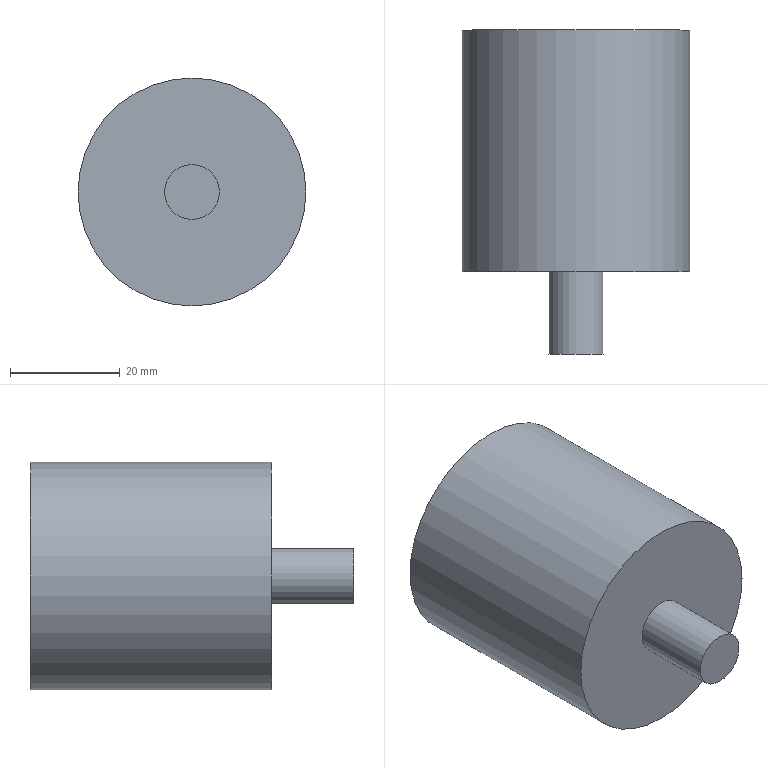Part | STEP file | 冲床-300配套压波_id286_x_t | 1 solid | 5 faces | box 41.5 x 59 x 41.5 mm | volume 60695 mm3 | plane 3 | cylinder 2 | commonest cylinder face diameters 10 x1 41.5 x1
STEP:
#1=CARTESIAN_POINT('',(1130.,22.,181.5));
#2=VERTEX_POINT('',#1);
#3=CARTESIAN_POINT('',(1130.,22.,160.75));
#4=DIRECTION('',(0.,-1.,0.));
#5=DIRECTION('',(0.,0.,1.));
#6=AXIS2_PLACEMENT_3D('',#3,#4,#5);
#7=CIRCLE('',#6,20.75);
#8=EDGE_CURVE('',#2,#2,#7,.T.);
#9=ORIENTED_EDGE('',*,*,#8,.F.);
#10=EDGE_LOOP('',(#9));
#11=FACE_OUTER_BOUND('',#10,.T.);
#12=CARTESIAN_POINT('',(1130.,22.,110.));
#13=DIRECTION('',(0.,1.,0.));
#14=DIRECTION('',(0.,0.,1.));
#15=AXIS2_PLACEMENT_3D('',#12,#13,#14);
#16=PLANE('',#15);
#17=ADVANCED_FACE('',(#11),#16,.T.);
#18=CARTESIAN_POINT('',(1130.,-22.,181.5));
#19=VERTEX_POINT('',#18);
#20=CARTESIAN_POINT('',(1130.,-22.,160.75));
#21=DIRECTION('',(0.,1.,0.));
#22=DIRECTION('',(0.,0.,1.));
#23=AXIS2_PLACEMENT_3D('',#20,#21,#22);
#24=CIRCLE('',#23,20.75);
#25=EDGE_CURVE('',#19,#19,#24,.T.);
#26=ORIENTED_EDGE('',*,*,#25,.T.);
#27=EDGE_LOOP('',(#26));
#28=FACE_BOUND('',#27,.T.);
#29=ORIENTED_EDGE('',*,*,#8,.T.);
#30=EDGE_LOOP('',(#29));
#31=FACE_BOUND('',#30,.T.);
#32=CARTESIAN_POINT('',(1130.,-20.,160.75));
#33=DIRECTION('',(0.,1.,0.));
#34=DIRECTION('',(0.,0.,1.));
#35=AXIS2_PLACEMENT_3D('',#32,#33,#34);
#36=CYLINDRICAL_SURFACE('',#35,20.75);
#37=ADVANCED_FACE('',(#28,#31),#36,.T.);
#38=CARTESIAN_POINT('',(1130.,-22.,155.75));
#39=VERTEX_POINT('',#38);
#40=CARTESIAN_POINT('',(1130.,-22.,160.75));
#41=DIRECTION('',(0.,-1.,0.));
#42=DIRECTION('',(0.,0.,-1.));
#43=AXIS2_PLACEMENT_3D('',#40,#41,#42);
#44=CIRCLE('',#43,5.);
#45=EDGE_CURVE('',#39,#39,#44,.T.);
#46=ORIENTED_EDGE('',*,*,#45,.F.);
#47=EDGE_LOOP('',(#46));
#48=FACE_BOUND('',#47,.T.);
#49=ORIENTED_EDGE('',*,*,#25,.F.);
#50=EDGE_LOOP('',(#49));
#51=FACE_BOUND('',#50,.T.);
#52=CARTESIAN_POINT('',(1130.,-22.,160.75));
#53=DIRECTION('',(0.,1.,0.));
#54=DIRECTION('',(0.,0.,1.));
#55=AXIS2_PLACEMENT_3D('',#52,#53,#54);
#56=PLANE('',#55);
#57=ADVANCED_FACE('',(#48,#51),#56,.F.);
#58=CARTESIAN_POINT('',(1130.,-37.,165.75));
#59=VERTEX_POINT('',#58);
#60=CARTESIAN_POINT('',(1130.,-37.,160.75));
#61=DIRECTION('',(0.,-1.,0.));
#62=DIRECTION('',(0.,0.,1.));
#63=AXIS2_PLACEMENT_3D('',#60,#61,#62);
#64=CIRCLE('',#63,5.);
#65=EDGE_CURVE('',#59,#59,#64,.T.);
#66=ORIENTED_EDGE('',*,*,#65,.F.);
#67=EDGE_LOOP('',(#66));
#68=FACE_BOUND('',#67,.T.);
#69=ORIENTED_EDGE('',*,*,#45,.T.);
#70=EDGE_LOOP('',(#69));
#71=FACE_BOUND('',#70,.T.);
#72=CARTESIAN_POINT('',(1130.,-55.,160.75));
#73=DIRECTION('',(0.,1.,0.));
#74=DIRECTION('',(0.,0.,1.));
#75=AXIS2_PLACEMENT_3D('',#72,#73,#74);
#76=CYLINDRICAL_SURFACE('',#75,5.);
#77=ADVANCED_FACE('',(#68,#71),#76,.T.);
#78=ORIENTED_EDGE('',*,*,#65,.T.);
#79=EDGE_LOOP('',(#78));
#80=FACE_OUTER_BOUND('',#79,.T.);
#81=CARTESIAN_POINT('',(1130.,-37.,160.75));
#82=DIRECTION('',(0.,1.,0.));
#83=DIRECTION('',(0.,0.,1.));
#84=AXIS2_PLACEMENT_3D('',#81,#82,#83);
#85=PLANE('',#84);
#86=ADVANCED_FACE('',(#80),#85,.F.);
#87=CLOSED_SHELL('',(#17,#37,#57,#77,#86));
#88=MANIFOLD_SOLID_BREP('',#87);
#89=(LENGTH_UNIT()NAMED_UNIT(*)SI_UNIT(.MILLI.,.METRE.));
#90=UNCERTAINTY_MEASURE_WITH_UNIT(LENGTH_MEASURE(0.00002),#89,'','');
#91=(NAMED_UNIT(*)PLANE_ANGLE_UNIT()SI_UNIT($,.RADIAN.));
#92=PLANE_ANGLE_MEASURE_WITH_UNIT(PLANE_ANGLE_MEASURE(0.01745),#91);
#93=DIMENSIONAL_EXPONENTS(0.,0.,0.,0.,0.,0.,0.);
#94=(CONVERSION_BASED_UNIT('DEGREE',#92)NAMED_UNIT(#93)PLANE_ANGLE_UNIT());
#95=(NAMED_UNIT(*)SI_UNIT($,.STERADIAN.)SOLID_ANGLE_UNIT());
#96=(GEOMETRIC_REPRESENTATION_CONTEXT(3)GLOBAL_UNCERTAINTY_ASSIGNED_CONTEXT((#90))GLOBAL_UNIT_ASSIGNED_CONTEXT((#89,#94,#95))REPRESENTATION_CONTEXT('',''));
#97=ADVANCED_BREP_SHAPE_REPRESENTATION('',(#88),#96);